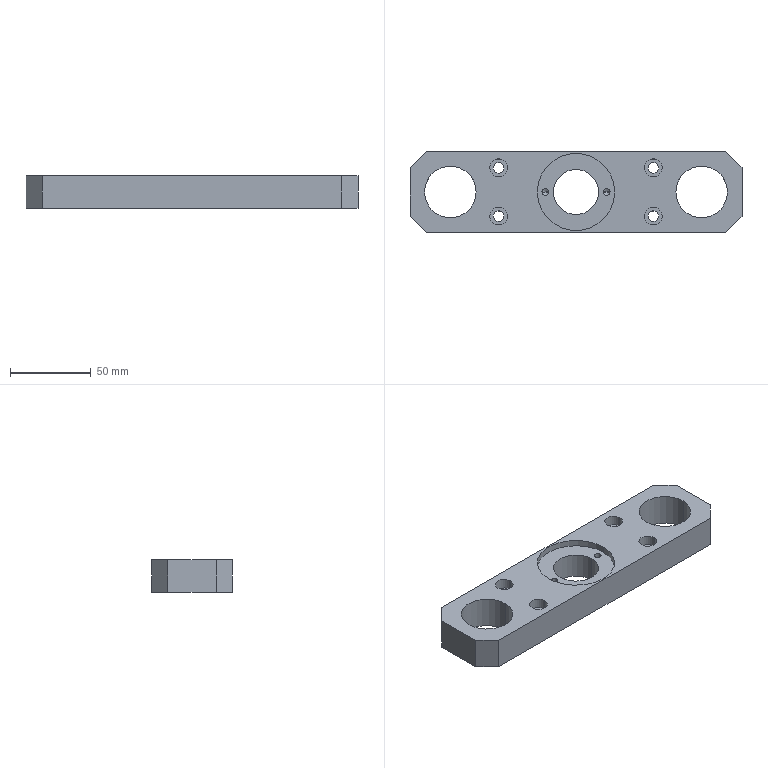Part | STEP file | BU-A05 | 1 solid | 47 faces | box 206 x 50 x 20 mm | volume 148133 mm3 | cylinder 28 | plane 15 | cone 4 | commonest cylinder face diameters 6.5 x8 11 x8 4.2 x4 32 x4 28 x2 48 x2